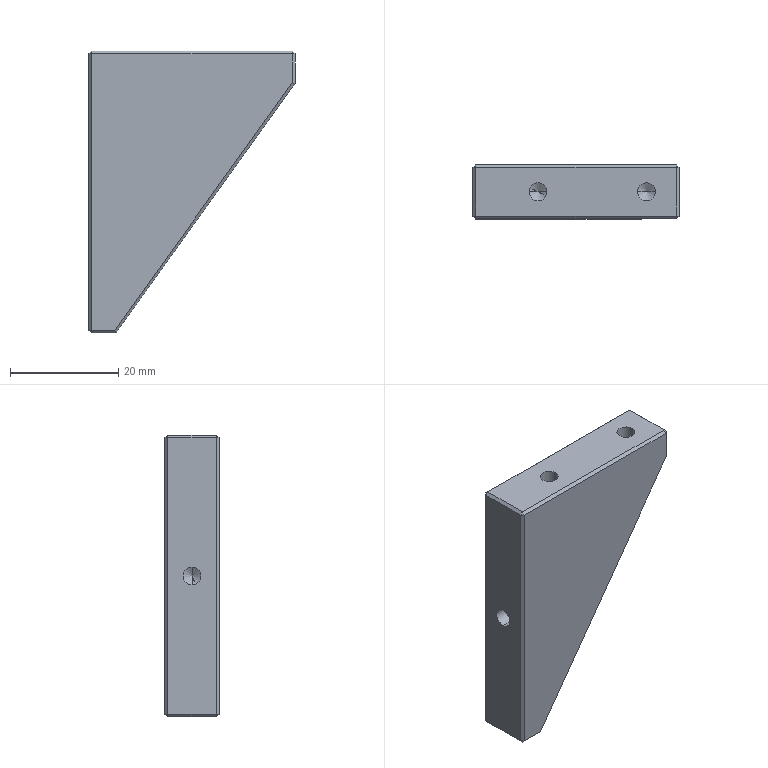Part | STEP file | ND25021-01-JDKM-30-TL | 1 solid | 38 faces | box 38 x 10 x 52 mm | volume 11845 mm3 | plane 26 | cylinder 6 | cone 6 | commonest cylinder face diameters 3.3 x6